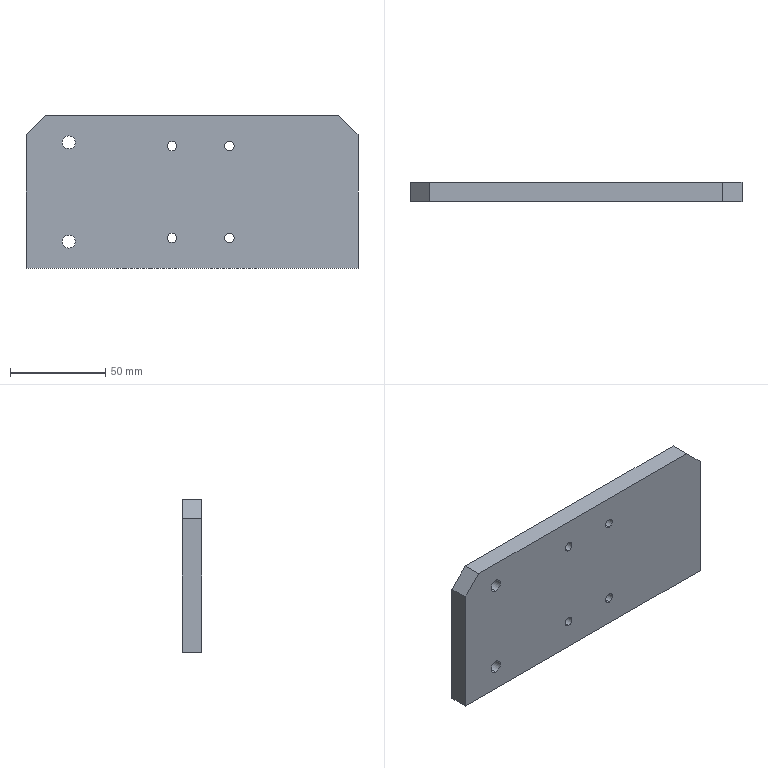Part | STEP file | X77-04204 | 1 solid | 20 faces | box 174 x 10 x 80 mm | volume 136688 mm3 | cylinder 12 | plane 8 | commonest cylinder face diameters 5 x8 6.8 x4
STEP:
#1=CARTESIAN_POINT('',(250.227,-17.171,62.6));
#2=VERTEX_POINT('',#1);
#3=CARTESIAN_POINT('',(250.227,-17.171,69.4));
#4=VERTEX_POINT('',#3);
#5=CARTESIAN_POINT('',(250.227,-17.171,66.));
#6=DIRECTION('',(0.,1.,0.));
#7=DIRECTION('',(-1.,0.,0.));
#8=AXIS2_PLACEMENT_3D('',#5,#6,#7);
#9=CIRCLE('',#8,3.4);
#10=EDGE_CURVE('',#2,#4,#9,.T.);
#11=ORIENTED_EDGE('',*,*,#10,.F.);
#12=CARTESIAN_POINT('',(250.227,-7.171,62.6));
#13=VERTEX_POINT('',#12);
#14=CARTESIAN_POINT('',(250.227,-7.171,62.6));
#15=DIRECTION('',(0.,1.,0.));
#16=VECTOR('',#15,1000.);
#17=LINE('',#14,#16);
#18=EDGE_CURVE('',#2,#13,#17,.T.);
#19=ORIENTED_EDGE('',*,*,#18,.T.);
#20=CARTESIAN_POINT('',(250.227,-7.171,69.4));
#21=VERTEX_POINT('',#20);
#22=CARTESIAN_POINT('',(250.227,-7.171,66.));
#23=DIRECTION('',(0.,1.,0.));
#24=DIRECTION('',(0.,0.,1.));
#25=AXIS2_PLACEMENT_3D('',#22,#23,#24);
#26=CIRCLE('',#25,3.4);
#27=EDGE_CURVE('',#13,#21,#26,.T.);
#28=ORIENTED_EDGE('',*,*,#27,.T.);
#29=CARTESIAN_POINT('',(250.227,-7.171,69.4));
#30=DIRECTION('',(0.,1.,0.));
#31=VECTOR('',#30,1000.);
#32=LINE('',#29,#31);
#33=EDGE_CURVE('',#4,#21,#32,.T.);
#34=ORIENTED_EDGE('',*,*,#33,.F.);
#35=EDGE_LOOP('',(#11,#19,#28,#34));
#36=FACE_OUTER_BOUND('',#35,.T.);
#37=CARTESIAN_POINT('',(250.227,-7.171,66.));
#38=DIRECTION('',(0.,1.,0.));
#39=DIRECTION('',(0.,0.,1.));
#40=AXIS2_PLACEMENT_3D('',#37,#38,#39);
#41=CYLINDRICAL_SURFACE('',#40,3.4);
#42=ADVANCED_FACE('',(#36),#41,.F.);
#43=CARTESIAN_POINT('',(250.227,-17.171,10.6));
#44=VERTEX_POINT('',#43);
#45=CARTESIAN_POINT('',(250.227,-17.171,17.4));
#46=VERTEX_POINT('',#45);
#47=CARTESIAN_POINT('',(250.227,-17.171,14.));
#48=DIRECTION('',(0.,1.,0.));
#49=DIRECTION('',(-1.,0.,0.));
#50=AXIS2_PLACEMENT_3D('',#47,#48,#49);
#51=CIRCLE('',#50,3.4);
#52=EDGE_CURVE('',#44,#46,#51,.T.);
#53=ORIENTED_EDGE('',*,*,#52,.F.);
#54=CARTESIAN_POINT('',(250.227,-7.171,10.6));
#55=VERTEX_POINT('',#54);
#56=CARTESIAN_POINT('',(250.227,-7.171,10.6));
#57=DIRECTION('',(0.,1.,0.));
#58=VECTOR('',#57,1000.);
#59=LINE('',#56,#58);
#60=EDGE_CURVE('',#44,#55,#59,.T.);
#61=ORIENTED_EDGE('',*,*,#60,.T.);
#62=CARTESIAN_POINT('',(250.227,-7.171,17.4));
#63=VERTEX_POINT('',#62);
#64=CARTESIAN_POINT('',(250.227,-7.171,14.));
#65=DIRECTION('',(0.,1.,0.));
#66=DIRECTION('',(0.,0.,1.));
#67=AXIS2_PLACEMENT_3D('',#64,#65,#66);
#68=CIRCLE('',#67,3.4);
#69=EDGE_CURVE('',#55,#63,#68,.T.);
#70=ORIENTED_EDGE('',*,*,#69,.T.);
#71=CARTESIAN_POINT('',(250.227,-7.171,17.4));
#72=DIRECTION('',(0.,1.,0.));
#73=VECTOR('',#72,1000.);
#74=LINE('',#71,#73);
#75=EDGE_CURVE('',#46,#63,#74,.T.);
#76=ORIENTED_EDGE('',*,*,#75,.F.);
#77=EDGE_LOOP('',(#53,#61,#70,#76));
#78=FACE_OUTER_BOUND('',#77,.T.);
#79=CARTESIAN_POINT('',(250.227,-7.171,14.));
#80=DIRECTION('',(0.,1.,0.));
#81=DIRECTION('',(0.,0.,1.));
#82=AXIS2_PLACEMENT_3D('',#79,#80,#81);
#83=CYLINDRICAL_SURFACE('',#82,3.4);
#84=ADVANCED_FACE('',(#78),#83,.F.);
#85=CARTESIAN_POINT('',(304.275,-17.171,61.5));
#86=VERTEX_POINT('',#85);
#87=CARTESIAN_POINT('',(304.275,-17.171,66.5));
#88=VERTEX_POINT('',#87);
#89=CARTESIAN_POINT('',(304.275,-17.171,64.));
#90=DIRECTION('',(0.,1.,0.));
#91=DIRECTION('',(-1.,0.,0.));
#92=AXIS2_PLACEMENT_3D('',#89,#90,#91);
#93=CIRCLE('',#92,2.5);
#94=EDGE_CURVE('',#86,#88,#93,.T.);
#95=ORIENTED_EDGE('',*,*,#94,.F.);
#96=CARTESIAN_POINT('',(304.275,-7.171,61.5));
#97=VERTEX_POINT('',#96);
#98=CARTESIAN_POINT('',(304.275,-7.171,61.5));
#99=DIRECTION('',(0.,1.,0.));
#100=VECTOR('',#99,1000.);
#101=LINE('',#98,#100);
#102=EDGE_CURVE('',#86,#97,#101,.T.);
#103=ORIENTED_EDGE('',*,*,#102,.T.);
#104=CARTESIAN_POINT('',(304.275,-7.171,66.5));
#105=VERTEX_POINT('',#104);
#106=CARTESIAN_POINT('',(304.275,-7.171,64.));
#107=DIRECTION('',(0.,1.,0.));
#108=DIRECTION('',(0.,0.,1.));
#109=AXIS2_PLACEMENT_3D('',#106,#107,#108);
#110=CIRCLE('',#109,2.5);
#111=EDGE_CURVE('',#97,#105,#110,.T.);
#112=ORIENTED_EDGE('',*,*,#111,.T.);
#113=CARTESIAN_POINT('',(304.275,-7.171,66.5));
#114=DIRECTION('',(0.,1.,0.));
#115=VECTOR('',#114,1000.);
#116=LINE('',#113,#115);
#117=EDGE_CURVE('',#88,#105,#116,.T.);
#118=ORIENTED_EDGE('',*,*,#117,.F.);
#119=EDGE_LOOP('',(#95,#103,#112,#118));
#120=FACE_OUTER_BOUND('',#119,.T.);
#121=CARTESIAN_POINT('',(304.275,-7.171,64.));
#122=DIRECTION('',(0.,1.,0.));
#123=DIRECTION('',(0.,0.,1.));
#124=AXIS2_PLACEMENT_3D('',#121,#122,#123);
#125=CYLINDRICAL_SURFACE('',#124,2.5);
#126=ADVANCED_FACE('',(#120),#125,.F.);
#127=CARTESIAN_POINT('',(304.275,-17.171,13.5));
#128=VERTEX_POINT('',#127);
#129=CARTESIAN_POINT('',(304.275,-17.171,18.5));
#130=VERTEX_POINT('',#129);
#131=CARTESIAN_POINT('',(304.275,-17.171,16.));
#132=DIRECTION('',(0.,1.,0.));
#133=DIRECTION('',(-1.,0.,0.));
#134=AXIS2_PLACEMENT_3D('',#131,#132,#133);
#135=CIRCLE('',#134,2.5);
#136=EDGE_CURVE('',#128,#130,#135,.T.);
#137=ORIENTED_EDGE('',*,*,#136,.F.);
#138=CARTESIAN_POINT('',(304.275,-7.171,13.5));
#139=VERTEX_POINT('',#138);
#140=CARTESIAN_POINT('',(304.275,-7.171,13.5));
#141=DIRECTION('',(0.,1.,0.));
#142=VECTOR('',#141,1000.);
#143=LINE('',#140,#142);
#144=EDGE_CURVE('',#128,#139,#143,.T.);
#145=ORIENTED_EDGE('',*,*,#144,.T.);
#146=CARTESIAN_POINT('',(304.275,-7.171,18.5));
#147=VERTEX_POINT('',#146);
#148=CARTESIAN_POINT('',(304.275,-7.171,16.));
#149=DIRECTION('',(0.,1.,0.));
#150=DIRECTION('',(0.,0.,1.));
#151=AXIS2_PLACEMENT_3D('',#148,#149,#150);
#152=CIRCLE('',#151,2.5);
#153=EDGE_CURVE('',#139,#147,#152,.T.);
#154=ORIENTED_EDGE('',*,*,#153,.T.);
#155=CARTESIAN_POINT('',(304.275,-7.171,18.5));
#156=DIRECTION('',(0.,1.,0.));
#157=VECTOR('',#156,1000.);
#158=LINE('',#155,#157);
#159=EDGE_CURVE('',#130,#147,#158,.T.);
#160=ORIENTED_EDGE('',*,*,#159,.F.);
#161=EDGE_LOOP('',(#137,#145,#154,#160));
#162=FACE_OUTER_BOUND('',#161,.T.);
#163=CARTESIAN_POINT('',(304.275,-7.171,16.));
#164=DIRECTION('',(0.,1.,0.));
#165=DIRECTION('',(0.,0.,1.));
#166=AXIS2_PLACEMENT_3D('',#163,#164,#165);
#167=CYLINDRICAL_SURFACE('',#166,2.5);
#168=ADVANCED_FACE('',(#162),#167,.F.);
#169=CARTESIAN_POINT('',(334.275,-17.171,61.5));
#170=VERTEX_POINT('',#169);
#171=CARTESIAN_POINT('',(334.275,-17.171,66.5));
#172=VERTEX_POINT('',#171);
#173=CARTESIAN_POINT('',(334.275,-17.171,64.));
#174=DIRECTION('',(0.,1.,0.));
#175=DIRECTION('',(-1.,0.,0.));
#176=AXIS2_PLACEMENT_3D('',#173,#174,#175);
#177=CIRCLE('',#176,2.5);
#178=EDGE_CURVE('',#170,#172,#177,.T.);
#179=ORIENTED_EDGE('',*,*,#178,.F.);
#180=CARTESIAN_POINT('',(334.275,-7.171,61.5));
#181=VERTEX_POINT('',#180);
#182=CARTESIAN_POINT('',(334.275,-7.171,61.5));
#183=DIRECTION('',(0.,1.,0.));
#184=VECTOR('',#183,1000.);
#185=LINE('',#182,#184);
#186=EDGE_CURVE('',#170,#181,#185,.T.);
#187=ORIENTED_EDGE('',*,*,#186,.T.);
#188=CARTESIAN_POINT('',(334.275,-7.171,66.5));
#189=VERTEX_POINT('',#188);
#190=CARTESIAN_POINT('',(334.275,-7.171,64.));
#191=DIRECTION('',(0.,1.,0.));
#192=DIRECTION('',(0.,0.,1.));
#193=AXIS2_PLACEMENT_3D('',#190,#191,#192);
#194=CIRCLE('',#193,2.5);
#195=EDGE_CURVE('',#181,#189,#194,.T.);
#196=ORIENTED_EDGE('',*,*,#195,.T.);
#197=CARTESIAN_POINT('',(334.275,-7.171,66.5));
#198=DIRECTION('',(0.,1.,0.));
#199=VECTOR('',#198,1000.);
#200=LINE('',#197,#199);
#201=EDGE_CURVE('',#172,#189,#200,.T.);
#202=ORIENTED_EDGE('',*,*,#201,.F.);
#203=EDGE_LOOP('',(#179,#187,#196,#202));
#204=FACE_OUTER_BOUND('',#203,.T.);
#205=CARTESIAN_POINT('',(334.275,-7.171,64.));
#206=DIRECTION('',(0.,1.,0.));
#207=DIRECTION('',(0.,0.,1.));
#208=AXIS2_PLACEMENT_3D('',#205,#206,#207);
#209=CYLINDRICAL_SURFACE('',#208,2.5);
#210=ADVANCED_FACE('',(#204),#209,.F.);
#211=CARTESIAN_POINT('',(334.275,-17.171,13.5));
#212=VERTEX_POINT('',#211);
#213=CARTESIAN_POINT('',(334.275,-17.171,18.5));
#214=VERTEX_POINT('',#213);
#215=CARTESIAN_POINT('',(334.275,-17.171,16.));
#216=DIRECTION('',(0.,1.,0.));
#217=DIRECTION('',(-1.,0.,0.));
#218=AXIS2_PLACEMENT_3D('',#215,#216,#217);
#219=CIRCLE('',#218,2.5);
#220=EDGE_CURVE('',#212,#214,#219,.T.);
#221=ORIENTED_EDGE('',*,*,#220,.F.);
#222=CARTESIAN_POINT('',(334.275,-7.171,13.5));
#223=VERTEX_POINT('',#222);
#224=CARTESIAN_POINT('',(334.275,-7.171,13.5));
#225=DIRECTION('',(0.,1.,0.));
#226=VECTOR('',#225,1000.);
#227=LINE('',#224,#226);
#228=EDGE_CURVE('',#212,#223,#227,.T.);
#229=ORIENTED_EDGE('',*,*,#228,.T.);
#230=CARTESIAN_POINT('',(334.275,-7.171,18.5));
#231=VERTEX_POINT('',#230);
#232=CARTESIAN_POINT('',(334.275,-7.171,16.));
#233=DIRECTION('',(0.,1.,0.));
#234=DIRECTION('',(0.,0.,1.));
#235=AXIS2_PLACEMENT_3D('',#232,#233,#234);
#236=CIRCLE('',#235,2.5);
#237=EDGE_CURVE('',#223,#231,#236,.T.);
#238=ORIENTED_EDGE('',*,*,#237,.T.);
#239=CARTESIAN_POINT('',(334.275,-7.171,18.5));
#240=DIRECTION('',(0.,1.,0.));
#241=VECTOR('',#240,1000.);
#242=LINE('',#239,#241);
#243=EDGE_CURVE('',#214,#231,#242,.T.);
#244=ORIENTED_EDGE('',*,*,#243,.F.);
#245=EDGE_LOOP('',(#221,#229,#238,#244));
#246=FACE_OUTER_BOUND('',#245,.T.);
#247=CARTESIAN_POINT('',(334.275,-7.171,16.));
#248=DIRECTION('',(0.,1.,0.));
#249=DIRECTION('',(0.,0.,1.));
#250=AXIS2_PLACEMENT_3D('',#247,#248,#249);
#251=CYLINDRICAL_SURFACE('',#250,2.5);
#252=ADVANCED_FACE('',(#246),#251,.F.);
#253=CARTESIAN_POINT('',(401.727,-7.171,70.));
#254=VERTEX_POINT('',#253);
#255=CARTESIAN_POINT('',(401.727,-7.171,0.));
#256=VERTEX_POINT('',#255);
#257=CARTESIAN_POINT('',(401.727,-7.171,80.));
#258=DIRECTION('',(0.,0.,-1.));
#259=VECTOR('',#258,1000.);
#260=LINE('',#257,#259);
#261=EDGE_CURVE('',#254,#256,#260,.T.);
#262=ORIENTED_EDGE('',*,*,#261,.F.);
#263=CARTESIAN_POINT('',(401.727,-17.171,70.));
#264=VERTEX_POINT('',#263);
#265=CARTESIAN_POINT('',(401.727,-7.171,70.));
#266=DIRECTION('',(0.,-1.,0.));
#267=VECTOR('',#266,1000.);
#268=LINE('',#265,#267);
#269=EDGE_CURVE('',#254,#264,#268,.T.);
#270=ORIENTED_EDGE('',*,*,#269,.T.);
#271=CARTESIAN_POINT('',(401.727,-17.171,0.));
#272=VERTEX_POINT('',#271);
#273=CARTESIAN_POINT('',(401.727,-17.171,80.));
#274=DIRECTION('',(0.,0.,-1.));
#275=VECTOR('',#274,1000.);
#276=LINE('',#273,#275);
#277=EDGE_CURVE('',#264,#272,#276,.T.);
#278=ORIENTED_EDGE('',*,*,#277,.T.);
#279=CARTESIAN_POINT('',(401.727,-7.171,0.));
#280=DIRECTION('',(0.,1.,0.));
#281=VECTOR('',#280,1000.);
#282=LINE('',#279,#281);
#283=EDGE_CURVE('',#272,#256,#282,.T.);
#284=ORIENTED_EDGE('',*,*,#283,.T.);
#285=EDGE_LOOP('',(#262,#270,#278,#284));
#286=FACE_OUTER_BOUND('',#285,.T.);
#287=CARTESIAN_POINT('',(401.727,-7.171,80.));
#288=DIRECTION('',(-1.,0.,0.));
#289=DIRECTION('',(0.,0.,1.));
#290=AXIS2_PLACEMENT_3D('',#287,#288,#289);
#291=PLANE('',#290);
#292=ADVANCED_FACE('',(#286),#291,.F.);
#293=CARTESIAN_POINT('',(250.227,-7.171,66.));
#294=DIRECTION('',(0.,1.,0.));
#295=DIRECTION('',(0.,0.,1.));
#296=AXIS2_PLACEMENT_3D('',#293,#294,#295);
#297=CIRCLE('',#296,3.4);
#298=EDGE_CURVE('',#21,#13,#297,.T.);
#299=ORIENTED_EDGE('',*,*,#298,.F.);
#300=ORIENTED_EDGE('',*,*,#27,.F.);
#301=EDGE_LOOP('',(#299,#300));
#302=FACE_BOUND('',#301,.T.);
#303=CARTESIAN_POINT('',(250.227,-7.171,14.));
#304=DIRECTION('',(0.,1.,0.));
#305=DIRECTION('',(0.,0.,1.));
#306=AXIS2_PLACEMENT_3D('',#303,#304,#305);
#307=CIRCLE('',#306,3.4);
#308=EDGE_CURVE('',#63,#55,#307,.T.);
#309=ORIENTED_EDGE('',*,*,#308,.F.);
#310=ORIENTED_EDGE('',*,*,#69,.F.);
#311=EDGE_LOOP('',(#309,#310));
#312=FACE_BOUND('',#311,.T.);
#313=CARTESIAN_POINT('',(304.275,-7.171,64.));
#314=DIRECTION('',(0.,1.,0.));
#315=DIRECTION('',(0.,0.,1.));
#316=AXIS2_PLACEMENT_3D('',#313,#314,#315);
#317=CIRCLE('',#316,2.5);
#318=EDGE_CURVE('',#105,#97,#317,.T.);
#319=ORIENTED_EDGE('',*,*,#318,.F.);
#320=ORIENTED_EDGE('',*,*,#111,.F.);
#321=EDGE_LOOP('',(#319,#320));
#322=FACE_BOUND('',#321,.T.);
#323=CARTESIAN_POINT('',(304.275,-7.171,16.));
#324=DIRECTION('',(0.,1.,0.));
#325=DIRECTION('',(0.,0.,1.));
#326=AXIS2_PLACEMENT_3D('',#323,#324,#325);
#327=CIRCLE('',#326,2.5);
#328=EDGE_CURVE('',#147,#139,#327,.T.);
#329=ORIENTED_EDGE('',*,*,#328,.F.);
#330=ORIENTED_EDGE('',*,*,#153,.F.);
#331=EDGE_LOOP('',(#329,#330));
#332=FACE_BOUND('',#331,.T.);
#333=CARTESIAN_POINT('',(334.275,-7.171,64.));
#334=DIRECTION('',(0.,1.,0.));
#335=DIRECTION('',(0.,0.,1.));
#336=AXIS2_PLACEMENT_3D('',#333,#334,#335);
#337=CIRCLE('',#336,2.5);
#338=EDGE_CURVE('',#189,#181,#337,.T.);
#339=ORIENTED_EDGE('',*,*,#338,.F.);
#340=ORIENTED_EDGE('',*,*,#195,.F.);
#341=EDGE_LOOP('',(#339,#340));
#342=FACE_BOUND('',#341,.T.);
#343=CARTESIAN_POINT('',(334.275,-7.171,16.));
#344=DIRECTION('',(0.,1.,0.));
#345=DIRECTION('',(0.,0.,1.));
#346=AXIS2_PLACEMENT_3D('',#343,#344,#345);
#347=CIRCLE('',#346,2.5);
#348=EDGE_CURVE('',#231,#223,#347,.T.);
#349=ORIENTED_EDGE('',*,*,#348,.F.);
#350=ORIENTED_EDGE('',*,*,#237,.F.);
#351=EDGE_LOOP('',(#349,#350));
#352=FACE_BOUND('',#351,.T.);
#353=CARTESIAN_POINT('',(391.727,-7.171,80.));
#354=VERTEX_POINT('',#353);
#355=CARTESIAN_POINT('',(237.727,-7.171,80.));
#356=VERTEX_POINT('',#355);
#357=CARTESIAN_POINT('',(401.727,-7.171,80.));
#358=DIRECTION('',(-1.,0.,0.));
#359=VECTOR('',#358,1000.);
#360=LINE('',#357,#359);
#361=EDGE_CURVE('',#354,#356,#360,.T.);
#362=ORIENTED_EDGE('',*,*,#361,.F.);
#363=CARTESIAN_POINT('',(391.727,-7.171,80.));
#364=DIRECTION('',(0.7071,0.,-0.7071));
#365=VECTOR('',#364,1000.);
#366=LINE('',#363,#365);
#367=EDGE_CURVE('',#354,#254,#366,.T.);
#368=ORIENTED_EDGE('',*,*,#367,.T.);
#369=ORIENTED_EDGE('',*,*,#261,.T.);
#370=CARTESIAN_POINT('',(227.727,-7.171,0.));
#371=VERTEX_POINT('',#370);
#372=CARTESIAN_POINT('',(401.727,-7.171,0.));
#373=DIRECTION('',(-1.,0.,0.));
#374=VECTOR('',#373,1000.);
#375=LINE('',#372,#374);
#376=EDGE_CURVE('',#256,#371,#375,.T.);
#377=ORIENTED_EDGE('',*,*,#376,.T.);
#378=CARTESIAN_POINT('',(227.727,-7.171,70.));
#379=VERTEX_POINT('',#378);
#380=CARTESIAN_POINT('',(227.727,-7.171,80.));
#381=DIRECTION('',(0.,0.,-1.));
#382=VECTOR('',#381,1000.);
#383=LINE('',#380,#382);
#384=EDGE_CURVE('',#379,#371,#383,.T.);
#385=ORIENTED_EDGE('',*,*,#384,.F.);
#386=CARTESIAN_POINT('',(237.727,-7.171,80.));
#387=DIRECTION('',(0.7071,0.,0.7071));
#388=VECTOR('',#387,1000.);
#389=LINE('',#386,#388);
#390=EDGE_CURVE('',#379,#356,#389,.T.);
#391=ORIENTED_EDGE('',*,*,#390,.T.);
#392=EDGE_LOOP('',(#362,#368,#369,#377,#385,#391));
#393=FACE_OUTER_BOUND('',#392,.T.);
#394=CARTESIAN_POINT('',(401.727,-7.171,80.));
#395=DIRECTION('',(0.,-1.,0.));
#396=DIRECTION('',(1.,0.,0.));
#397=AXIS2_PLACEMENT_3D('',#394,#395,#396);
#398=PLANE('',#397);
#399=ADVANCED_FACE('',(#302,#312,#322,#332,#342,#352,#393),#398,.F.);
#400=CARTESIAN_POINT('',(227.727,-17.171,70.));
#401=VERTEX_POINT('',#400);
#402=CARTESIAN_POINT('',(227.727,-17.171,0.));
#403=VERTEX_POINT('',#402);
#404=CARTESIAN_POINT('',(227.727,-17.171,80.));
#405=DIRECTION('',(0.,0.,-1.));
#406=VECTOR('',#405,1000.);
#407=LINE('',#404,#406);
#408=EDGE_CURVE('',#401,#403,#407,.T.);
#409=ORIENTED_EDGE('',*,*,#408,.F.);
#410=CARTESIAN_POINT('',(227.727,-7.171,70.));
#411=DIRECTION('',(0.,1.,0.));
#412=VECTOR('',#411,1000.);
#413=LINE('',#410,#412);
#414=EDGE_CURVE('',#401,#379,#413,.T.);
#415=ORIENTED_EDGE('',*,*,#414,.T.);
#416=ORIENTED_EDGE('',*,*,#384,.T.);
#417=CARTESIAN_POINT('',(227.727,-7.171,0.));
#418=DIRECTION('',(0.,-1.,0.));
#419=VECTOR('',#418,1000.);
#420=LINE('',#417,#419);
#421=EDGE_CURVE('',#371,#403,#420,.T.);
#422=ORIENTED_EDGE('',*,*,#421,.T.);
#423=EDGE_LOOP('',(#409,#415,#416,#422));
#424=FACE_OUTER_BOUND('',#423,.T.);
#425=CARTESIAN_POINT('',(227.727,-7.171,80.));
#426=DIRECTION('',(1.,0.,0.));
#427=DIRECTION('',(0.,0.,-1.));
#428=AXIS2_PLACEMENT_3D('',#425,#426,#427);
#429=PLANE('',#428);
#430=ADVANCED_FACE('',(#424),#429,.F.);
#431=CARTESIAN_POINT('',(250.227,-17.171,66.));
#432=DIRECTION('',(0.,1.,0.));
#433=DIRECTION('',(-1.,0.,0.));
#434=AXIS2_PLACEMENT_3D('',#431,#432,#433);
#435=CIRCLE('',#434,3.4);
#436=EDGE_CURVE('',#4,#2,#435,.T.);
#437=ORIENTED_EDGE('',*,*,#436,.T.);
#438=ORIENTED_EDGE('',*,*,#10,.T.);
#439=EDGE_LOOP('',(#437,#438));
#440=FACE_BOUND('',#439,.T.);
#441=CARTESIAN_POINT('',(250.227,-17.171,14.));
#442=DIRECTION('',(0.,1.,0.));
#443=DIRECTION('',(-1.,0.,0.));
#444=AXIS2_PLACEMENT_3D('',#441,#442,#443);
#445=CIRCLE('',#444,3.4);
#446=EDGE_CURVE('',#46,#44,#445,.T.);
#447=ORIENTED_EDGE('',*,*,#446,.T.);
#448=ORIENTED_EDGE('',*,*,#52,.T.);
#449=EDGE_LOOP('',(#447,#448));
#450=FACE_BOUND('',#449,.T.);
#451=CARTESIAN_POINT('',(304.275,-17.171,64.));
#452=DIRECTION('',(0.,1.,0.));
#453=DIRECTION('',(-1.,0.,0.));
#454=AXIS2_PLACEMENT_3D('',#451,#452,#453);
#455=CIRCLE('',#454,2.5);
#456=EDGE_CURVE('',#88,#86,#455,.T.);
#457=ORIENTED_EDGE('',*,*,#456,.T.);
#458=ORIENTED_EDGE('',*,*,#94,.T.);
#459=EDGE_LOOP('',(#457,#458));
#460=FACE_BOUND('',#459,.T.);
#461=CARTESIAN_POINT('',(304.275,-17.171,16.));
#462=DIRECTION('',(0.,1.,0.));
#463=DIRECTION('',(-1.,0.,0.));
#464=AXIS2_PLACEMENT_3D('',#461,#462,#463);
#465=CIRCLE('',#464,2.5);
#466=EDGE_CURVE('',#130,#128,#465,.T.);
#467=ORIENTED_EDGE('',*,*,#466,.T.);
#468=ORIENTED_EDGE('',*,*,#136,.T.);
#469=EDGE_LOOP('',(#467,#468));
#470=FACE_BOUND('',#469,.T.);
#471=CARTESIAN_POINT('',(334.275,-17.171,64.));
#472=DIRECTION('',(0.,1.,0.));
#473=DIRECTION('',(-1.,0.,0.));
#474=AXIS2_PLACEMENT_3D('',#471,#472,#473);
#475=CIRCLE('',#474,2.5);
#476=EDGE_CURVE('',#172,#170,#475,.T.);
#477=ORIENTED_EDGE('',*,*,#476,.T.);
#478=ORIENTED_EDGE('',*,*,#178,.T.);
#479=EDGE_LOOP('',(#477,#478));
#480=FACE_BOUND('',#479,.T.);
#481=CARTESIAN_POINT('',(334.275,-17.171,16.));
#482=DIRECTION('',(0.,1.,0.));
#483=DIRECTION('',(-1.,0.,0.));
#484=AXIS2_PLACEMENT_3D('',#481,#482,#483);
#485=CIRCLE('',#484,2.5);
#486=EDGE_CURVE('',#214,#212,#485,.T.);
#487=ORIENTED_EDGE('',*,*,#486,.T.);
#488=ORIENTED_EDGE('',*,*,#220,.T.);
#489=EDGE_LOOP('',(#487,#488));
#490=FACE_BOUND('',#489,.T.);
#491=ORIENTED_EDGE('',*,*,#277,.F.);
#492=CARTESIAN_POINT('',(391.727,-17.171,80.));
#493=VERTEX_POINT('',#492);
#494=CARTESIAN_POINT('',(391.727,-17.171,80.));
#495=DIRECTION('',(-0.7071,0.,0.7071));
#496=VECTOR('',#495,1000.);
#497=LINE('',#494,#496);
#498=EDGE_CURVE('',#264,#493,#497,.T.);
#499=ORIENTED_EDGE('',*,*,#498,.T.);
#500=CARTESIAN_POINT('',(237.727,-17.171,80.));
#501=VERTEX_POINT('',#500);
#502=CARTESIAN_POINT('',(401.727,-17.171,80.));
#503=DIRECTION('',(1.,0.,0.));
#504=VECTOR('',#503,1000.);
#505=LINE('',#502,#504);
#506=EDGE_CURVE('',#501,#493,#505,.T.);
#507=ORIENTED_EDGE('',*,*,#506,.F.);
#508=CARTESIAN_POINT('',(237.727,-17.171,80.));
#509=DIRECTION('',(-0.7071,0.,-0.7071));
#510=VECTOR('',#509,1000.);
#511=LINE('',#508,#510);
#512=EDGE_CURVE('',#501,#401,#511,.T.);
#513=ORIENTED_EDGE('',*,*,#512,.T.);
#514=ORIENTED_EDGE('',*,*,#408,.T.);
#515=CARTESIAN_POINT('',(401.727,-17.171,0.));
#516=DIRECTION('',(1.,0.,0.));
#517=VECTOR('',#516,1000.);
#518=LINE('',#515,#517);
#519=EDGE_CURVE('',#403,#272,#518,.T.);
#520=ORIENTED_EDGE('',*,*,#519,.T.);
#521=EDGE_LOOP('',(#491,#499,#507,#513,#514,#520));
#522=FACE_OUTER_BOUND('',#521,.T.);
#523=CARTESIAN_POINT('',(401.727,-17.171,80.));
#524=DIRECTION('',(0.,1.,0.));
#525=DIRECTION('',(-1.,0.,0.));
#526=AXIS2_PLACEMENT_3D('',#523,#524,#525);
#527=PLANE('',#526);
#528=ADVANCED_FACE('',(#440,#450,#460,#470,#480,#490,#522),#527,.F.);
#529=ORIENTED_EDGE('',*,*,#506,.T.);
#530=CARTESIAN_POINT('',(391.727,-17.171,80.));
#531=DIRECTION('',(0.,1.,0.));
#532=VECTOR('',#531,1000.);
#533=LINE('',#530,#532);
#534=EDGE_CURVE('',#493,#354,#533,.T.);
#535=ORIENTED_EDGE('',*,*,#534,.T.);
#536=ORIENTED_EDGE('',*,*,#361,.T.);
#537=CARTESIAN_POINT('',(237.727,-17.171,80.));
#538=DIRECTION('',(0.,-1.,0.));
#539=VECTOR('',#538,1000.);
#540=LINE('',#537,#539);
#541=EDGE_CURVE('',#356,#501,#540,.T.);
#542=ORIENTED_EDGE('',*,*,#541,.T.);
#543=EDGE_LOOP('',(#529,#535,#536,#542));
#544=FACE_OUTER_BOUND('',#543,.T.);
#545=CARTESIAN_POINT('',(401.727,-17.171,80.));
#546=DIRECTION('',(0.,0.,-1.));
#547=DIRECTION('',(-1.,0.,0.));
#548=AXIS2_PLACEMENT_3D('',#545,#546,#547);
#549=PLANE('',#548);
#550=ADVANCED_FACE('',(#544),#549,.F.);
#551=ORIENTED_EDGE('',*,*,#283,.F.);
#552=ORIENTED_EDGE('',*,*,#519,.F.);
#553=ORIENTED_EDGE('',*,*,#421,.F.);
#554=ORIENTED_EDGE('',*,*,#376,.F.);
#555=EDGE_LOOP('',(#551,#552,#553,#554));
#556=FACE_OUTER_BOUND('',#555,.T.);
#557=CARTESIAN_POINT('',(401.727,-17.171,0.));
#558=DIRECTION('',(0.,0.,-1.));
#559=DIRECTION('',(-1.,0.,0.));
#560=AXIS2_PLACEMENT_3D('',#557,#558,#559);
#561=PLANE('',#560);
#562=ADVANCED_FACE('',(#556),#561,.T.);
#563=ORIENTED_EDGE('',*,*,#228,.F.);
#564=ORIENTED_EDGE('',*,*,#486,.F.);
#565=ORIENTED_EDGE('',*,*,#243,.T.);
#566=ORIENTED_EDGE('',*,*,#348,.T.);
#567=EDGE_LOOP('',(#563,#564,#565,#566));
#568=FACE_OUTER_BOUND('',#567,.T.);
#569=CARTESIAN_POINT('',(334.275,-7.171,16.));
#570=DIRECTION('',(0.,1.,0.));
#571=DIRECTION('',(0.,0.,1.));
#572=AXIS2_PLACEMENT_3D('',#569,#570,#571);
#573=CYLINDRICAL_SURFACE('',#572,2.5);
#574=ADVANCED_FACE('',(#568),#573,.F.);
#575=ORIENTED_EDGE('',*,*,#186,.F.);
#576=ORIENTED_EDGE('',*,*,#476,.F.);
#577=ORIENTED_EDGE('',*,*,#201,.T.);
#578=ORIENTED_EDGE('',*,*,#338,.T.);
#579=EDGE_LOOP('',(#575,#576,#577,#578));
#580=FACE_OUTER_BOUND('',#579,.T.);
#581=CARTESIAN_POINT('',(334.275,-7.171,64.));
#582=DIRECTION('',(0.,1.,0.));
#583=DIRECTION('',(0.,0.,1.));
#584=AXIS2_PLACEMENT_3D('',#581,#582,#583);
#585=CYLINDRICAL_SURFACE('',#584,2.5);
#586=ADVANCED_FACE('',(#580),#585,.F.);
#587=ORIENTED_EDGE('',*,*,#144,.F.);
#588=ORIENTED_EDGE('',*,*,#466,.F.);
#589=ORIENTED_EDGE('',*,*,#159,.T.);
#590=ORIENTED_EDGE('',*,*,#328,.T.);
#591=EDGE_LOOP('',(#587,#588,#589,#590));
#592=FACE_OUTER_BOUND('',#591,.T.);
#593=CARTESIAN_POINT('',(304.275,-7.171,16.));
#594=DIRECTION('',(0.,1.,0.));
#595=DIRECTION('',(0.,0.,1.));
#596=AXIS2_PLACEMENT_3D('',#593,#594,#595);
#597=CYLINDRICAL_SURFACE('',#596,2.5);
#598=ADVANCED_FACE('',(#592),#597,.F.);
#599=ORIENTED_EDGE('',*,*,#102,.F.);
#600=ORIENTED_EDGE('',*,*,#456,.F.);
#601=ORIENTED_EDGE('',*,*,#117,.T.);
#602=ORIENTED_EDGE('',*,*,#318,.T.);
#603=EDGE_LOOP('',(#599,#600,#601,#602));
#604=FACE_OUTER_BOUND('',#603,.T.);
#605=CARTESIAN_POINT('',(304.275,-7.171,64.));
#606=DIRECTION('',(0.,1.,0.));
#607=DIRECTION('',(0.,0.,1.));
#608=AXIS2_PLACEMENT_3D('',#605,#606,#607);
#609=CYLINDRICAL_SURFACE('',#608,2.5);
#610=ADVANCED_FACE('',(#604),#609,.F.);
#611=ORIENTED_EDGE('',*,*,#60,.F.);
#612=ORIENTED_EDGE('',*,*,#446,.F.);
#613=ORIENTED_EDGE('',*,*,#75,.T.);
#614=ORIENTED_EDGE('',*,*,#308,.T.);
#615=EDGE_LOOP('',(#611,#612,#613,#614));
#616=FACE_OUTER_BOUND('',#615,.T.);
#617=CARTESIAN_POINT('',(250.227,-7.171,14.));
#618=DIRECTION('',(0.,1.,0.));
#619=DIRECTION('',(0.,0.,1.));
#620=AXIS2_PLACEMENT_3D('',#617,#618,#619);
#621=CYLINDRICAL_SURFACE('',#620,3.4);
#622=ADVANCED_FACE('',(#616),#621,.F.);
#623=ORIENTED_EDGE('',*,*,#18,.F.);
#624=ORIENTED_EDGE('',*,*,#436,.F.);
#625=ORIENTED_EDGE('',*,*,#33,.T.);
#626=ORIENTED_EDGE('',*,*,#298,.T.);
#627=EDGE_LOOP('',(#623,#624,#625,#626));
#628=FACE_OUTER_BOUND('',#627,.T.);
#629=CARTESIAN_POINT('',(250.227,-7.171,66.));
#630=DIRECTION('',(0.,1.,0.));
#631=DIRECTION('',(0.,0.,1.));
#632=AXIS2_PLACEMENT_3D('',#629,#630,#631);
#633=CYLINDRICAL_SURFACE('',#632,3.4);
#634=ADVANCED_FACE('',(#628),#633,.F.);
#635=ORIENTED_EDGE('',*,*,#498,.F.);
#636=ORIENTED_EDGE('',*,*,#269,.F.);
#637=ORIENTED_EDGE('',*,*,#367,.F.);
#638=ORIENTED_EDGE('',*,*,#534,.F.);
#639=EDGE_LOOP('',(#635,#636,#637,#638));
#640=FACE_OUTER_BOUND('',#639,.T.);
#641=CARTESIAN_POINT('',(391.727,-17.171,80.));
#642=DIRECTION('',(-0.7071,0.,-0.7071));
#643=DIRECTION('',(-0.7071,0.,0.7071));
#644=AXIS2_PLACEMENT_3D('',#641,#642,#643);
#645=PLANE('',#644);
#646=ADVANCED_FACE('',(#640),#645,.F.);
#647=ORIENTED_EDGE('',*,*,#390,.F.);
#648=ORIENTED_EDGE('',*,*,#414,.F.);
#649=ORIENTED_EDGE('',*,*,#512,.F.);
#650=ORIENTED_EDGE('',*,*,#541,.F.);
#651=EDGE_LOOP('',(#647,#648,#649,#650));
#652=FACE_OUTER_BOUND('',#651,.T.);
#653=CARTESIAN_POINT('',(237.727,-17.171,80.));
#654=DIRECTION('',(0.7071,0.,-0.7071));
#655=DIRECTION('',(-0.7071,0.,-0.7071));
#656=AXIS2_PLACEMENT_3D('',#653,#654,#655);
#657=PLANE('',#656);
#658=ADVANCED_FACE('',(#652),#657,.F.);
#659=CLOSED_SHELL('',(#42,#84,#126,#168,#210,#252,#292,#399,#430,#528,#550,#562,#574,#586,#598,#610,#622,#634,#646,#658));
#660=MANIFOLD_SOLID_BREP('',#659);
#661=CARTESIAN_POINT('',(0.,0.,0.));
#662=DIRECTION('',(0.,0.,1.));
#663=DIRECTION('',(1.,0.,0.));
#664=AXIS2_PLACEMENT_3D('',#661,#662,#663);
#665=(LENGTH_UNIT()NAMED_UNIT(*)SI_UNIT(.MILLI.,.METRE.));
#666=UNCERTAINTY_MEASURE_WITH_UNIT(LENGTH_MEASURE(0.00001),#665,'','');
#667=(NAMED_UNIT(*)PLANE_ANGLE_UNIT()SI_UNIT($,.RADIAN.));
#668=(NAMED_UNIT(*)SI_UNIT($,.STERADIAN.)SOLID_ANGLE_UNIT());
#669=(GEOMETRIC_REPRESENTATION_CONTEXT(3)GLOBAL_UNCERTAINTY_ASSIGNED_CONTEXT((#666))GLOBAL_UNIT_ASSIGNED_CONTEXT((#665,#667,#668))REPRESENTATION_CONTEXT('',''));
#670=ADVANCED_BREP_SHAPE_REPRESENTATION('',(#660,#664),#669);